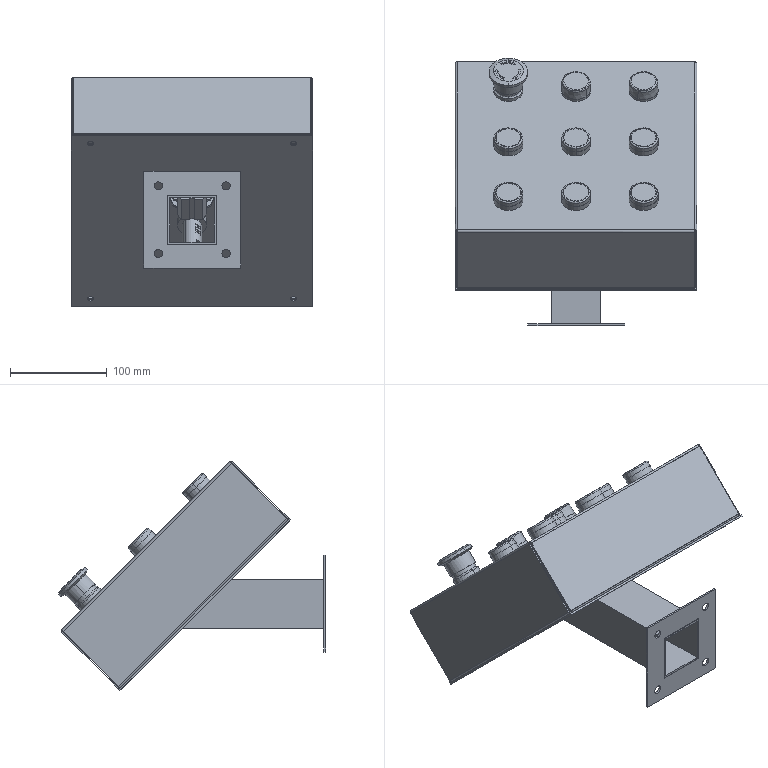Part | SolidWorks | 15 solids | 1142 faces | box 250 x 277.105 x 237.493 mm | volume 898997 mm3 | plane 769 | cylinder 279 | spline 86 | cone 8 | commonest cylinder face diameters 30 x99 22 x33 22.5 x18 4.5 x16 6.5 x16 25.7 x12